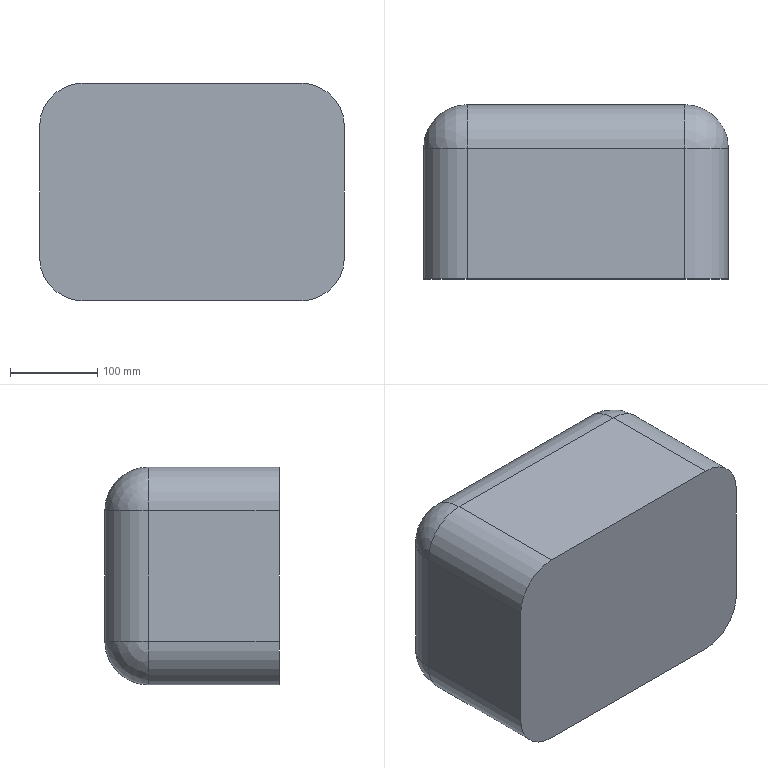Part | 1 solid | 18 faces | box 350 x 200 x 250 mm | volume 16510693 mm3 | cylinder 8 | plane 6 | sphere 4 | commonest cylinder face diameters 100 x8
STEP:
#1=CARTESIAN_POINT('',(175.,0.,-75.));
#2=VERTEX_POINT('',#1);
#3=CARTESIAN_POINT('',(175.,150.,-75.));
#4=VERTEX_POINT('',#3);
#5=CARTESIAN_POINT('',(175.,200.,-75.));
#6=DIRECTION('',(0.,1.,0.));
#7=VECTOR('',#6,1000.);
#8=LINE('',#5,#7);
#9=EDGE_CURVE('',#2,#4,#8,.T.);
#10=ORIENTED_EDGE('',*,*,#9,.T.);
#11=CARTESIAN_POINT('',(175.,150.,75.));
#12=VERTEX_POINT('',#11);
#13=CARTESIAN_POINT('',(175.,150.,75.));
#14=DIRECTION('',(0.,0.,1.));
#15=VECTOR('',#14,1000.);
#16=LINE('',#13,#15);
#17=EDGE_CURVE('',#4,#12,#16,.T.);
#18=ORIENTED_EDGE('',*,*,#17,.T.);
#19=CARTESIAN_POINT('',(175.,0.,75.));
#20=VERTEX_POINT('',#19);
#21=CARTESIAN_POINT('',(175.,200.,75.));
#22=DIRECTION('',(0.,-1.,0.));
#23=VECTOR('',#22,1000.);
#24=LINE('',#21,#23);
#25=EDGE_CURVE('',#12,#20,#24,.T.);
#26=ORIENTED_EDGE('',*,*,#25,.T.);
#27=CARTESIAN_POINT('',(175.,0.,-125.));
#28=DIRECTION('',(0.,0.,-1.));
#29=VECTOR('',#28,1000.);
#30=LINE('',#27,#29);
#31=EDGE_CURVE('',#20,#2,#30,.T.);
#32=ORIENTED_EDGE('',*,*,#31,.T.);
#33=EDGE_LOOP('',(#10,#18,#26,#32));
#34=FACE_OUTER_BOUND('',#33,.T.);
#35=CARTESIAN_POINT('',(175.,200.,-125.));
#36=DIRECTION('',(-1.,0.,0.));
#37=DIRECTION('',(0.,0.,1.));
#38=AXIS2_PLACEMENT_3D('',#35,#36,#37);
#39=PLANE('',#38);
#40=ADVANCED_FACE('',(#34),#39,.F.);
#41=CARTESIAN_POINT('',(-125.,0.,-125.));
#42=VERTEX_POINT('',#41);
#43=CARTESIAN_POINT('',(-125.,150.,-125.));
#44=VERTEX_POINT('',#43);
#45=CARTESIAN_POINT('',(-125.,200.,-125.));
#46=DIRECTION('',(0.,1.,0.));
#47=VECTOR('',#46,1000.);
#48=LINE('',#45,#47);
#49=EDGE_CURVE('',#42,#44,#48,.T.);
#50=ORIENTED_EDGE('',*,*,#49,.T.);
#51=CARTESIAN_POINT('',(125.,150.,-125.));
#52=VERTEX_POINT('',#51);
#53=CARTESIAN_POINT('',(125.,150.,-125.));
#54=DIRECTION('',(1.,0.,0.));
#55=VECTOR('',#54,1000.);
#56=LINE('',#53,#55);
#57=EDGE_CURVE('',#44,#52,#56,.T.);
#58=ORIENTED_EDGE('',*,*,#57,.T.);
#59=CARTESIAN_POINT('',(125.,0.,-125.));
#60=VERTEX_POINT('',#59);
#61=CARTESIAN_POINT('',(125.,200.,-125.));
#62=DIRECTION('',(0.,-1.,0.));
#63=VECTOR('',#62,1000.);
#64=LINE('',#61,#63);
#65=EDGE_CURVE('',#52,#60,#64,.T.);
#66=ORIENTED_EDGE('',*,*,#65,.T.);
#67=CARTESIAN_POINT('',(-175.,0.,-125.));
#68=DIRECTION('',(-1.,0.,0.));
#69=VECTOR('',#68,1000.);
#70=LINE('',#67,#69);
#71=EDGE_CURVE('',#60,#42,#70,.T.);
#72=ORIENTED_EDGE('',*,*,#71,.T.);
#73=EDGE_LOOP('',(#50,#58,#66,#72));
#74=FACE_OUTER_BOUND('',#73,.T.);
#75=CARTESIAN_POINT('',(-175.,200.,-125.));
#76=DIRECTION('',(0.,0.,1.));
#77=DIRECTION('',(1.,0.,0.));
#78=AXIS2_PLACEMENT_3D('',#75,#76,#77);
#79=PLANE('',#78);
#80=ADVANCED_FACE('',(#74),#79,.F.);
#81=CARTESIAN_POINT('',(-175.,0.,75.));
#82=VERTEX_POINT('',#81);
#83=CARTESIAN_POINT('',(-175.,150.,75.));
#84=VERTEX_POINT('',#83);
#85=CARTESIAN_POINT('',(-175.,200.,75.));
#86=DIRECTION('',(0.,1.,0.));
#87=VECTOR('',#86,1000.);
#88=LINE('',#85,#87);
#89=EDGE_CURVE('',#82,#84,#88,.T.);
#90=ORIENTED_EDGE('',*,*,#89,.T.);
#91=CARTESIAN_POINT('',(-175.,150.,-75.));
#92=VERTEX_POINT('',#91);
#93=CARTESIAN_POINT('',(-175.,150.,-75.));
#94=DIRECTION('',(0.,0.,-1.));
#95=VECTOR('',#94,1000.);
#96=LINE('',#93,#95);
#97=EDGE_CURVE('',#84,#92,#96,.T.);
#98=ORIENTED_EDGE('',*,*,#97,.T.);
#99=CARTESIAN_POINT('',(-175.,0.,-75.));
#100=VERTEX_POINT('',#99);
#101=CARTESIAN_POINT('',(-175.,200.,-75.));
#102=DIRECTION('',(0.,-1.,0.));
#103=VECTOR('',#102,1000.);
#104=LINE('',#101,#103);
#105=EDGE_CURVE('',#92,#100,#104,.T.);
#106=ORIENTED_EDGE('',*,*,#105,.T.);
#107=CARTESIAN_POINT('',(-175.,0.,-125.));
#108=DIRECTION('',(0.,0.,1.));
#109=VECTOR('',#108,1000.);
#110=LINE('',#107,#109);
#111=EDGE_CURVE('',#100,#82,#110,.T.);
#112=ORIENTED_EDGE('',*,*,#111,.T.);
#113=EDGE_LOOP('',(#90,#98,#106,#112));
#114=FACE_OUTER_BOUND('',#113,.T.);
#115=CARTESIAN_POINT('',(-175.,200.,-125.));
#116=DIRECTION('',(1.,0.,0.));
#117=DIRECTION('',(0.,0.,-1.));
#118=AXIS2_PLACEMENT_3D('',#115,#116,#117);
#119=PLANE('',#118);
#120=ADVANCED_FACE('',(#114),#119,.F.);
#121=CARTESIAN_POINT('',(125.,0.,125.));
#122=VERTEX_POINT('',#121);
#123=CARTESIAN_POINT('',(125.,150.,125.));
#124=VERTEX_POINT('',#123);
#125=CARTESIAN_POINT('',(125.,200.,125.));
#126=DIRECTION('',(0.,1.,0.));
#127=VECTOR('',#126,1000.);
#128=LINE('',#125,#127);
#129=EDGE_CURVE('',#122,#124,#128,.T.);
#130=ORIENTED_EDGE('',*,*,#129,.T.);
#131=CARTESIAN_POINT('',(-125.,150.,125.));
#132=VERTEX_POINT('',#131);
#133=CARTESIAN_POINT('',(-125.,150.,125.));
#134=DIRECTION('',(-1.,0.,0.));
#135=VECTOR('',#134,1000.);
#136=LINE('',#133,#135);
#137=EDGE_CURVE('',#124,#132,#136,.T.);
#138=ORIENTED_EDGE('',*,*,#137,.T.);
#139=CARTESIAN_POINT('',(-125.,0.,125.));
#140=VERTEX_POINT('',#139);
#141=CARTESIAN_POINT('',(-125.,200.,125.));
#142=DIRECTION('',(0.,-1.,0.));
#143=VECTOR('',#142,1000.);
#144=LINE('',#141,#143);
#145=EDGE_CURVE('',#132,#140,#144,.T.);
#146=ORIENTED_EDGE('',*,*,#145,.T.);
#147=CARTESIAN_POINT('',(-175.,0.,125.));
#148=DIRECTION('',(1.,0.,0.));
#149=VECTOR('',#148,1000.);
#150=LINE('',#147,#149);
#151=EDGE_CURVE('',#140,#122,#150,.T.);
#152=ORIENTED_EDGE('',*,*,#151,.T.);
#153=EDGE_LOOP('',(#130,#138,#146,#152));
#154=FACE_OUTER_BOUND('',#153,.T.);
#155=CARTESIAN_POINT('',(-175.,200.,125.));
#156=DIRECTION('',(0.,0.,-1.));
#157=DIRECTION('',(-1.,0.,0.));
#158=AXIS2_PLACEMENT_3D('',#155,#156,#157);
#159=PLANE('',#158);
#160=ADVANCED_FACE('',(#154),#159,.F.);
#161=CARTESIAN_POINT('',(-125.,200.,-75.));
#162=VERTEX_POINT('',#161);
#163=CARTESIAN_POINT('',(-125.,200.,75.));
#164=VERTEX_POINT('',#163);
#165=CARTESIAN_POINT('',(-125.,200.,75.));
#166=DIRECTION('',(0.,0.,1.));
#167=VECTOR('',#166,1000.);
#168=LINE('',#165,#167);
#169=EDGE_CURVE('',#162,#164,#168,.T.);
#170=ORIENTED_EDGE('',*,*,#169,.T.);
#171=CARTESIAN_POINT('',(125.,200.,75.));
#172=VERTEX_POINT('',#171);
#173=CARTESIAN_POINT('',(125.,200.,75.));
#174=DIRECTION('',(1.,0.,0.));
#175=VECTOR('',#174,1000.);
#176=LINE('',#173,#175);
#177=EDGE_CURVE('',#164,#172,#176,.T.);
#178=ORIENTED_EDGE('',*,*,#177,.T.);
#179=CARTESIAN_POINT('',(125.,200.,-75.));
#180=VERTEX_POINT('',#179);
#181=CARTESIAN_POINT('',(125.,200.,-75.));
#182=DIRECTION('',(0.,0.,-1.));
#183=VECTOR('',#182,1000.);
#184=LINE('',#181,#183);
#185=EDGE_CURVE('',#172,#180,#184,.T.);
#186=ORIENTED_EDGE('',*,*,#185,.T.);
#187=CARTESIAN_POINT('',(-125.,200.,-75.));
#188=DIRECTION('',(-1.,0.,0.));
#189=VECTOR('',#188,1000.);
#190=LINE('',#187,#189);
#191=EDGE_CURVE('',#180,#162,#190,.T.);
#192=ORIENTED_EDGE('',*,*,#191,.T.);
#193=EDGE_LOOP('',(#170,#178,#186,#192));
#194=FACE_OUTER_BOUND('',#193,.T.);
#195=CARTESIAN_POINT('',(0.,200.,0.));
#196=DIRECTION('',(0.,1.,0.));
#197=DIRECTION('',(0.,0.,1.));
#198=AXIS2_PLACEMENT_3D('',#195,#196,#197);
#199=PLANE('',#198);
#200=ADVANCED_FACE('',(#194),#199,.T.);
#201=ORIENTED_EDGE('',*,*,#71,.F.);
#202=CARTESIAN_POINT('',(125.,0.,-75.));
#203=DIRECTION('',(0.,-1.,0.));
#204=DIRECTION('',(0.,0.,1.));
#205=AXIS2_PLACEMENT_3D('',#202,#203,#204);
#206=CIRCLE('',#205,50.);
#207=EDGE_CURVE('',#60,#2,#206,.T.);
#208=ORIENTED_EDGE('',*,*,#207,.T.);
#209=ORIENTED_EDGE('',*,*,#31,.F.);
#210=CARTESIAN_POINT('',(125.,0.,75.));
#211=DIRECTION('',(0.,-1.,0.));
#212=DIRECTION('',(0.,0.,1.));
#213=AXIS2_PLACEMENT_3D('',#210,#211,#212);
#214=CIRCLE('',#213,50.);
#215=EDGE_CURVE('',#20,#122,#214,.T.);
#216=ORIENTED_EDGE('',*,*,#215,.T.);
#217=ORIENTED_EDGE('',*,*,#151,.F.);
#218=CARTESIAN_POINT('',(-125.,0.,75.));
#219=DIRECTION('',(0.,-1.,0.));
#220=DIRECTION('',(0.,0.,1.));
#221=AXIS2_PLACEMENT_3D('',#218,#219,#220);
#222=CIRCLE('',#221,50.);
#223=EDGE_CURVE('',#140,#82,#222,.T.);
#224=ORIENTED_EDGE('',*,*,#223,.T.);
#225=ORIENTED_EDGE('',*,*,#111,.F.);
#226=CARTESIAN_POINT('',(-125.,0.,-75.));
#227=DIRECTION('',(0.,-1.,0.));
#228=DIRECTION('',(0.,0.,1.));
#229=AXIS2_PLACEMENT_3D('',#226,#227,#228);
#230=CIRCLE('',#229,50.);
#231=EDGE_CURVE('',#100,#42,#230,.T.);
#232=ORIENTED_EDGE('',*,*,#231,.T.);
#233=EDGE_LOOP('',(#201,#208,#209,#216,#217,#224,#225,#232));
#234=FACE_OUTER_BOUND('',#233,.T.);
#235=CARTESIAN_POINT('',(0.,0.,0.));
#236=DIRECTION('',(0.,1.,0.));
#237=DIRECTION('',(0.,0.,1.));
#238=AXIS2_PLACEMENT_3D('',#235,#236,#237);
#239=PLANE('',#238);
#240=ADVANCED_FACE('',(#234),#239,.F.);
#241=ORIENTED_EDGE('',*,*,#65,.F.);
#242=CARTESIAN_POINT('',(125.,150.,-75.));
#243=DIRECTION('',(0.,-1.,0.));
#244=DIRECTION('',(0.,0.,-1.));
#245=AXIS2_PLACEMENT_3D('',#242,#243,#244);
#246=CIRCLE('',#245,50.);
#247=EDGE_CURVE('',#52,#4,#246,.T.);
#248=ORIENTED_EDGE('',*,*,#247,.T.);
#249=ORIENTED_EDGE('',*,*,#9,.F.);
#250=ORIENTED_EDGE('',*,*,#207,.F.);
#251=EDGE_LOOP('',(#241,#248,#249,#250));
#252=FACE_OUTER_BOUND('',#251,.T.);
#253=CARTESIAN_POINT('',(125.,200.,-75.));
#254=DIRECTION('',(0.,-1.,0.));
#255=DIRECTION('',(0.,0.,-1.));
#256=AXIS2_PLACEMENT_3D('',#253,#254,#255);
#257=CYLINDRICAL_SURFACE('',#256,50.);
#258=ADVANCED_FACE('',(#252),#257,.T.);
#259=ORIENTED_EDGE('',*,*,#25,.F.);
#260=CARTESIAN_POINT('',(125.,150.,75.));
#261=DIRECTION('',(0.,-1.,0.));
#262=DIRECTION('',(0.,0.,-1.));
#263=AXIS2_PLACEMENT_3D('',#260,#261,#262);
#264=CIRCLE('',#263,50.);
#265=EDGE_CURVE('',#12,#124,#264,.T.);
#266=ORIENTED_EDGE('',*,*,#265,.T.);
#267=ORIENTED_EDGE('',*,*,#129,.F.);
#268=ORIENTED_EDGE('',*,*,#215,.F.);
#269=EDGE_LOOP('',(#259,#266,#267,#268));
#270=FACE_OUTER_BOUND('',#269,.T.);
#271=CARTESIAN_POINT('',(125.,200.,75.));
#272=DIRECTION('',(0.,-1.,0.));
#273=DIRECTION('',(0.,0.,-1.));
#274=AXIS2_PLACEMENT_3D('',#271,#272,#273);
#275=CYLINDRICAL_SURFACE('',#274,50.);
#276=ADVANCED_FACE('',(#270),#275,.T.);
#277=ORIENTED_EDGE('',*,*,#105,.F.);
#278=CARTESIAN_POINT('',(-125.,150.,-75.));
#279=DIRECTION('',(0.,-1.,0.));
#280=DIRECTION('',(0.,0.,-1.));
#281=AXIS2_PLACEMENT_3D('',#278,#279,#280);
#282=CIRCLE('',#281,50.);
#283=EDGE_CURVE('',#92,#44,#282,.T.);
#284=ORIENTED_EDGE('',*,*,#283,.T.);
#285=ORIENTED_EDGE('',*,*,#49,.F.);
#286=ORIENTED_EDGE('',*,*,#231,.F.);
#287=EDGE_LOOP('',(#277,#284,#285,#286));
#288=FACE_OUTER_BOUND('',#287,.T.);
#289=CARTESIAN_POINT('',(-125.,200.,-75.));
#290=DIRECTION('',(0.,-1.,0.));
#291=DIRECTION('',(0.,0.,-1.));
#292=AXIS2_PLACEMENT_3D('',#289,#290,#291);
#293=CYLINDRICAL_SURFACE('',#292,50.);
#294=ADVANCED_FACE('',(#288),#293,.T.);
#295=ORIENTED_EDGE('',*,*,#145,.F.);
#296=CARTESIAN_POINT('',(-125.,150.,75.));
#297=DIRECTION('',(0.,-1.,0.));
#298=DIRECTION('',(0.,0.,-1.));
#299=AXIS2_PLACEMENT_3D('',#296,#297,#298);
#300=CIRCLE('',#299,50.);
#301=EDGE_CURVE('',#132,#84,#300,.T.);
#302=ORIENTED_EDGE('',*,*,#301,.T.);
#303=ORIENTED_EDGE('',*,*,#89,.F.);
#304=ORIENTED_EDGE('',*,*,#223,.F.);
#305=EDGE_LOOP('',(#295,#302,#303,#304));
#306=FACE_OUTER_BOUND('',#305,.T.);
#307=CARTESIAN_POINT('',(-125.,200.,75.));
#308=DIRECTION('',(0.,-1.,0.));
#309=DIRECTION('',(0.,0.,-1.));
#310=AXIS2_PLACEMENT_3D('',#307,#308,#309);
#311=CYLINDRICAL_SURFACE('',#310,50.);
#312=ADVANCED_FACE('',(#306),#311,.T.);
#313=CARTESIAN_POINT('',(-125.,150.,-75.));
#314=DIRECTION('',(1.,0.,0.));
#315=DIRECTION('',(0.,0.,-1.));
#316=AXIS2_PLACEMENT_3D('',#313,#314,#315);
#317=CIRCLE('',#316,50.);
#318=EDGE_CURVE('',#44,#162,#317,.T.);
#319=ORIENTED_EDGE('',*,*,#318,.F.);
#320=ORIENTED_EDGE('',*,*,#283,.F.);
#321=CARTESIAN_POINT('',(-125.,150.,-75.));
#322=DIRECTION('',(0.,0.,1.));
#323=DIRECTION('',(1.,0.,0.));
#324=AXIS2_PLACEMENT_3D('',#321,#322,#323);
#325=CIRCLE('',#324,50.);
#326=EDGE_CURVE('',#162,#92,#325,.T.);
#327=ORIENTED_EDGE('',*,*,#326,.F.);
#328=EDGE_LOOP('',(#319,#320,#327));
#329=FACE_OUTER_BOUND('',#328,.T.);
#330=CARTESIAN_POINT('',(-125.,150.,-75.));
#331=DIRECTION('',(1.,0.,0.));
#332=DIRECTION('',(0.,0.,1.));
#333=AXIS2_PLACEMENT_3D('',#330,#331,#332);
#334=SPHERICAL_SURFACE('',#333,50.);
#335=ADVANCED_FACE('',(#329),#334,.T.);
#336=ORIENTED_EDGE('',*,*,#326,.T.);
#337=ORIENTED_EDGE('',*,*,#97,.F.);
#338=CARTESIAN_POINT('',(-125.,150.,75.));
#339=DIRECTION('',(0.,0.,1.));
#340=DIRECTION('',(1.,0.,0.));
#341=AXIS2_PLACEMENT_3D('',#338,#339,#340);
#342=CIRCLE('',#341,50.);
#343=EDGE_CURVE('',#164,#84,#342,.T.);
#344=ORIENTED_EDGE('',*,*,#343,.F.);
#345=ORIENTED_EDGE('',*,*,#169,.F.);
#346=EDGE_LOOP('',(#336,#337,#344,#345));
#347=FACE_OUTER_BOUND('',#346,.T.);
#348=CARTESIAN_POINT('',(-125.,150.,0.));
#349=DIRECTION('',(0.,0.,-1.));
#350=DIRECTION('',(-1.,0.,0.));
#351=AXIS2_PLACEMENT_3D('',#348,#349,#350);
#352=CYLINDRICAL_SURFACE('',#351,50.);
#353=ADVANCED_FACE('',(#347),#352,.T.);
#354=ORIENTED_EDGE('',*,*,#318,.T.);
#355=ORIENTED_EDGE('',*,*,#191,.F.);
#356=CARTESIAN_POINT('',(125.,150.,-75.));
#357=DIRECTION('',(1.,0.,0.));
#358=DIRECTION('',(0.,0.,-1.));
#359=AXIS2_PLACEMENT_3D('',#356,#357,#358);
#360=CIRCLE('',#359,50.);
#361=EDGE_CURVE('',#52,#180,#360,.T.);
#362=ORIENTED_EDGE('',*,*,#361,.F.);
#363=ORIENTED_EDGE('',*,*,#57,.F.);
#364=EDGE_LOOP('',(#354,#355,#362,#363));
#365=FACE_OUTER_BOUND('',#364,.T.);
#366=CARTESIAN_POINT('',(0.,150.,-75.));
#367=DIRECTION('',(1.,0.,0.));
#368=DIRECTION('',(0.,0.,-1.));
#369=AXIS2_PLACEMENT_3D('',#366,#367,#368);
#370=CYLINDRICAL_SURFACE('',#369,50.);
#371=ADVANCED_FACE('',(#365),#370,.T.);
#372=ORIENTED_EDGE('',*,*,#343,.T.);
#373=ORIENTED_EDGE('',*,*,#301,.F.);
#374=CARTESIAN_POINT('',(-125.,150.,75.));
#375=DIRECTION('',(1.,0.,0.));
#376=DIRECTION('',(0.,0.,-1.));
#377=AXIS2_PLACEMENT_3D('',#374,#375,#376);
#378=CIRCLE('',#377,50.);
#379=EDGE_CURVE('',#164,#132,#378,.T.);
#380=ORIENTED_EDGE('',*,*,#379,.F.);
#381=EDGE_LOOP('',(#372,#373,#380));
#382=FACE_OUTER_BOUND('',#381,.T.);
#383=CARTESIAN_POINT('',(-125.,150.,75.));
#384=DIRECTION('',(1.,0.,0.));
#385=DIRECTION('',(0.,0.,1.));
#386=AXIS2_PLACEMENT_3D('',#383,#384,#385);
#387=SPHERICAL_SURFACE('',#386,50.);
#388=ADVANCED_FACE('',(#382),#387,.T.);
#389=ORIENTED_EDGE('',*,*,#247,.F.);
#390=ORIENTED_EDGE('',*,*,#361,.T.);
#391=CARTESIAN_POINT('',(125.,150.,-75.));
#392=DIRECTION('',(0.,0.,1.));
#393=DIRECTION('',(1.,0.,0.));
#394=AXIS2_PLACEMENT_3D('',#391,#392,#393);
#395=CIRCLE('',#394,50.);
#396=EDGE_CURVE('',#4,#180,#395,.T.);
#397=ORIENTED_EDGE('',*,*,#396,.F.);
#398=EDGE_LOOP('',(#389,#390,#397));
#399=FACE_OUTER_BOUND('',#398,.T.);
#400=CARTESIAN_POINT('',(125.,150.,-75.));
#401=DIRECTION('',(1.,0.,0.));
#402=DIRECTION('',(0.,0.,1.));
#403=AXIS2_PLACEMENT_3D('',#400,#401,#402);
#404=SPHERICAL_SURFACE('',#403,50.);
#405=ADVANCED_FACE('',(#399),#404,.T.);
#406=ORIENTED_EDGE('',*,*,#379,.T.);
#407=ORIENTED_EDGE('',*,*,#137,.F.);
#408=CARTESIAN_POINT('',(125.,150.,75.));
#409=DIRECTION('',(1.,0.,0.));
#410=DIRECTION('',(0.,0.,-1.));
#411=AXIS2_PLACEMENT_3D('',#408,#409,#410);
#412=CIRCLE('',#411,50.);
#413=EDGE_CURVE('',#172,#124,#412,.T.);
#414=ORIENTED_EDGE('',*,*,#413,.F.);
#415=ORIENTED_EDGE('',*,*,#177,.F.);
#416=EDGE_LOOP('',(#406,#407,#414,#415));
#417=FACE_OUTER_BOUND('',#416,.T.);
#418=CARTESIAN_POINT('',(0.,150.,75.));
#419=DIRECTION('',(-1.,0.,0.));
#420=DIRECTION('',(0.,0.,1.));
#421=AXIS2_PLACEMENT_3D('',#418,#419,#420);
#422=CYLINDRICAL_SURFACE('',#421,50.);
#423=ADVANCED_FACE('',(#417),#422,.T.);
#424=ORIENTED_EDGE('',*,*,#396,.T.);
#425=ORIENTED_EDGE('',*,*,#185,.F.);
#426=CARTESIAN_POINT('',(125.,150.,75.));
#427=DIRECTION('',(0.,0.,1.));
#428=DIRECTION('',(1.,0.,0.));
#429=AXIS2_PLACEMENT_3D('',#426,#427,#428);
#430=CIRCLE('',#429,50.);
#431=EDGE_CURVE('',#12,#172,#430,.T.);
#432=ORIENTED_EDGE('',*,*,#431,.F.);
#433=ORIENTED_EDGE('',*,*,#17,.F.);
#434=EDGE_LOOP('',(#424,#425,#432,#433));
#435=FACE_OUTER_BOUND('',#434,.T.);
#436=CARTESIAN_POINT('',(125.,150.,0.));
#437=DIRECTION('',(0.,0.,1.));
#438=DIRECTION('',(1.,0.,0.));
#439=AXIS2_PLACEMENT_3D('',#436,#437,#438);
#440=CYLINDRICAL_SURFACE('',#439,50.);
#441=ADVANCED_FACE('',(#435),#440,.T.);
#442=ORIENTED_EDGE('',*,*,#413,.T.);
#443=ORIENTED_EDGE('',*,*,#265,.F.);
#444=ORIENTED_EDGE('',*,*,#431,.T.);
#445=EDGE_LOOP('',(#442,#443,#444));
#446=FACE_OUTER_BOUND('',#445,.T.);
#447=CARTESIAN_POINT('',(125.,150.,75.));
#448=DIRECTION('',(1.,0.,0.));
#449=DIRECTION('',(0.,0.,1.));
#450=AXIS2_PLACEMENT_3D('',#447,#448,#449);
#451=SPHERICAL_SURFACE('',#450,50.);
#452=ADVANCED_FACE('',(#446),#451,.T.);
#453=CLOSED_SHELL('',(#40,#80,#120,#160,#200,#240,#258,#276,#294,#312,#335,#353,#371,#388,#405,#423,#441,#452));
#454=MANIFOLD_SOLID_BREP('',#453);
#455=CARTESIAN_POINT('',(0.,0.,0.));
#456=DIRECTION('',(0.,0.,1.));
#457=DIRECTION('',(1.,0.,0.));
#458=AXIS2_PLACEMENT_3D('',#455,#456,#457);
#459=(LENGTH_UNIT()NAMED_UNIT(*)SI_UNIT(.MILLI.,.METRE.));
#460=UNCERTAINTY_MEASURE_WITH_UNIT(LENGTH_MEASURE(0.00001),#459,'','');
#461=(NAMED_UNIT(*)PLANE_ANGLE_UNIT()SI_UNIT($,.RADIAN.));
#462=(NAMED_UNIT(*)SI_UNIT($,.STERADIAN.)SOLID_ANGLE_UNIT());
#463=(GEOMETRIC_REPRESENTATION_CONTEXT(3)GLOBAL_UNCERTAINTY_ASSIGNED_CONTEXT((#460))GLOBAL_UNIT_ASSIGNED_CONTEXT((#459,#461,#462))REPRESENTATION_CONTEXT('',''));
#464=ADVANCED_BREP_SHAPE_REPRESENTATION('',(#454,#458),#463);